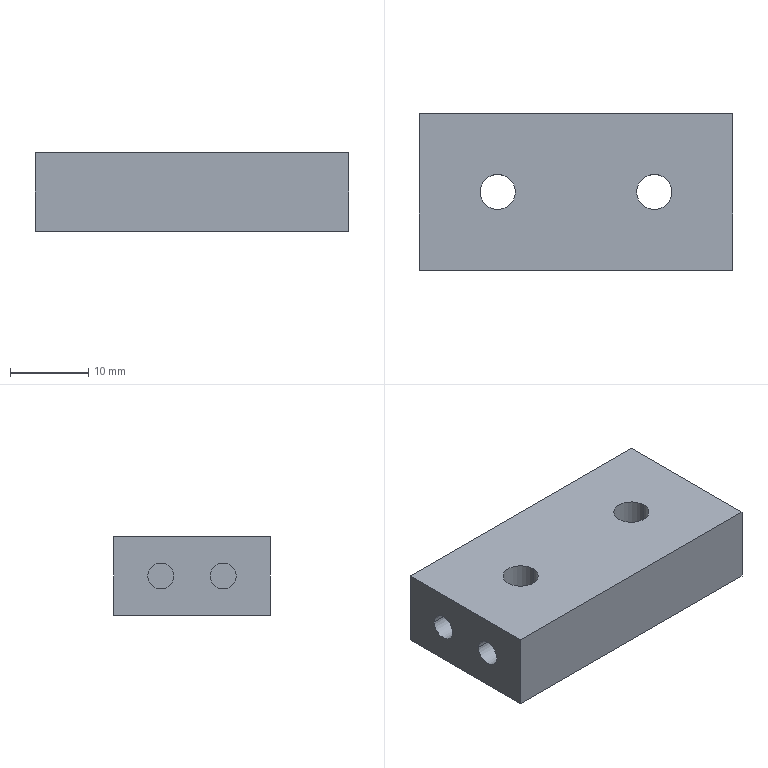Part | SolidWorks | features ICE 2, Extrusion 1 | 1 solid | 22 faces | box 40 x 20 x 10 mm | volume 7288 mm3 | cylinder 12 | plane 10 | commonest cylinder face diameters 3.3 x8 4.5 x4
STEP:
#1=CARTESIAN_POINT('',(9.151,4.195,6.65));
#2=VERTEX_POINT('',#1);
#3=CARTESIAN_POINT('',(9.151,4.195,3.35));
#4=VERTEX_POINT('',#3);
#5=CARTESIAN_POINT('',(9.151,4.195,5.));
#6=DIRECTION('',(1.,0.,0.));
#7=DIRECTION('',(0.,0.,-1.));
#8=AXIS2_PLACEMENT_3D('',#5,#6,#7);
#9=CIRCLE('',#8,1.65);
#10=EDGE_CURVE('',#2,#4,#9,.T.);
#11=ORIENTED_EDGE('',*,*,#10,.F.);
#12=CARTESIAN_POINT('',(20.651,4.195,6.65));
#13=VERTEX_POINT('',#12);
#14=CARTESIAN_POINT('',(9.151,4.195,6.65));
#15=DIRECTION('',(1.,0.,0.));
#16=VECTOR('',#15,1000.);
#17=LINE('',#14,#16);
#18=EDGE_CURVE('',#2,#13,#17,.T.);
#19=ORIENTED_EDGE('',*,*,#18,.T.);
#20=CARTESIAN_POINT('',(20.651,4.195,3.35));
#21=VERTEX_POINT('',#20);
#22=CARTESIAN_POINT('',(20.651,4.195,5.));
#23=DIRECTION('',(1.,0.,0.));
#24=DIRECTION('',(0.,0.,-1.));
#25=AXIS2_PLACEMENT_3D('',#22,#23,#24);
#26=CIRCLE('',#25,1.65);
#27=EDGE_CURVE('',#13,#21,#26,.T.);
#28=ORIENTED_EDGE('',*,*,#27,.T.);
#29=CARTESIAN_POINT('',(9.151,4.195,3.35));
#30=DIRECTION('',(1.,0.,0.));
#31=VECTOR('',#30,1000.);
#32=LINE('',#29,#31);
#33=EDGE_CURVE('',#4,#21,#32,.T.);
#34=ORIENTED_EDGE('',*,*,#33,.F.);
#35=EDGE_LOOP('',(#11,#19,#28,#34));
#36=FACE_OUTER_BOUND('',#35,.T.);
#37=CARTESIAN_POINT('',(9.151,4.195,5.));
#38=DIRECTION('',(1.,0.,0.));
#39=DIRECTION('',(0.,0.,-1.));
#40=AXIS2_PLACEMENT_3D('',#37,#38,#39);
#41=CYLINDRICAL_SURFACE('',#40,1.65);
#42=ADVANCED_FACE('',(#36),#41,.F.);
#43=CARTESIAN_POINT('',(9.151,-3.805,6.65));
#44=VERTEX_POINT('',#43);
#45=CARTESIAN_POINT('',(9.151,-3.805,3.35));
#46=VERTEX_POINT('',#45);
#47=CARTESIAN_POINT('',(9.151,-3.805,5.));
#48=DIRECTION('',(1.,0.,0.));
#49=DIRECTION('',(0.,0.,-1.));
#50=AXIS2_PLACEMENT_3D('',#47,#48,#49);
#51=CIRCLE('',#50,1.65);
#52=EDGE_CURVE('',#44,#46,#51,.T.);
#53=ORIENTED_EDGE('',*,*,#52,.F.);
#54=CARTESIAN_POINT('',(20.651,-3.805,6.65));
#55=VERTEX_POINT('',#54);
#56=CARTESIAN_POINT('',(9.151,-3.805,6.65));
#57=DIRECTION('',(1.,0.,0.));
#58=VECTOR('',#57,1000.);
#59=LINE('',#56,#58);
#60=EDGE_CURVE('',#44,#55,#59,.T.);
#61=ORIENTED_EDGE('',*,*,#60,.T.);
#62=CARTESIAN_POINT('',(20.651,-3.805,3.35));
#63=VERTEX_POINT('',#62);
#64=CARTESIAN_POINT('',(20.651,-3.805,5.));
#65=DIRECTION('',(1.,0.,0.));
#66=DIRECTION('',(0.,0.,-1.));
#67=AXIS2_PLACEMENT_3D('',#64,#65,#66);
#68=CIRCLE('',#67,1.65);
#69=EDGE_CURVE('',#55,#63,#68,.T.);
#70=ORIENTED_EDGE('',*,*,#69,.T.);
#71=CARTESIAN_POINT('',(9.151,-3.805,3.35));
#72=DIRECTION('',(1.,0.,0.));
#73=VECTOR('',#72,1000.);
#74=LINE('',#71,#73);
#75=EDGE_CURVE('',#46,#63,#74,.T.);
#76=ORIENTED_EDGE('',*,*,#75,.F.);
#77=EDGE_LOOP('',(#53,#61,#70,#76));
#78=FACE_OUTER_BOUND('',#77,.T.);
#79=CARTESIAN_POINT('',(9.151,-3.805,5.));
#80=DIRECTION('',(1.,0.,0.));
#81=DIRECTION('',(0.,0.,-1.));
#82=AXIS2_PLACEMENT_3D('',#79,#80,#81);
#83=CYLINDRICAL_SURFACE('',#82,1.65);
#84=ADVANCED_FACE('',(#78),#83,.F.);
#85=CARTESIAN_POINT('',(-7.849,5.845,5.));
#86=VERTEX_POINT('',#85);
#87=CARTESIAN_POINT('',(-7.849,2.545,5.));
#88=VERTEX_POINT('',#87);
#89=CARTESIAN_POINT('',(-7.849,4.195,5.));
#90=DIRECTION('',(-1.,0.,0.));
#91=DIRECTION('',(0.,-1.,0.));
#92=AXIS2_PLACEMENT_3D('',#89,#90,#91);
#93=CIRCLE('',#92,1.65);
#94=EDGE_CURVE('',#86,#88,#93,.T.);
#95=ORIENTED_EDGE('',*,*,#94,.F.);
#96=CARTESIAN_POINT('',(-19.349,5.845,5.));
#97=VERTEX_POINT('',#96);
#98=CARTESIAN_POINT('',(-7.849,5.845,5.));
#99=DIRECTION('',(-1.,0.,0.));
#100=VECTOR('',#99,1000.);
#101=LINE('',#98,#100);
#102=EDGE_CURVE('',#86,#97,#101,.T.);
#103=ORIENTED_EDGE('',*,*,#102,.T.);
#104=CARTESIAN_POINT('',(-19.349,2.545,5.));
#105=VERTEX_POINT('',#104);
#106=CARTESIAN_POINT('',(-19.349,4.195,5.));
#107=DIRECTION('',(-1.,0.,0.));
#108=DIRECTION('',(0.,-1.,0.));
#109=AXIS2_PLACEMENT_3D('',#106,#107,#108);
#110=CIRCLE('',#109,1.65);
#111=EDGE_CURVE('',#97,#105,#110,.T.);
#112=ORIENTED_EDGE('',*,*,#111,.T.);
#113=CARTESIAN_POINT('',(-7.849,2.545,5.));
#114=DIRECTION('',(-1.,0.,0.));
#115=VECTOR('',#114,1000.);
#116=LINE('',#113,#115);
#117=EDGE_CURVE('',#88,#105,#116,.T.);
#118=ORIENTED_EDGE('',*,*,#117,.F.);
#119=EDGE_LOOP('',(#95,#103,#112,#118));
#120=FACE_OUTER_BOUND('',#119,.T.);
#121=CARTESIAN_POINT('',(-7.849,4.195,5.));
#122=DIRECTION('',(-1.,0.,0.));
#123=DIRECTION('',(0.,-1.,0.));
#124=AXIS2_PLACEMENT_3D('',#121,#122,#123);
#125=CYLINDRICAL_SURFACE('',#124,1.65);
#126=ADVANCED_FACE('',(#120),#125,.F.);
#127=CARTESIAN_POINT('',(-7.849,-2.155,5.));
#128=VERTEX_POINT('',#127);
#129=CARTESIAN_POINT('',(-7.849,-5.455,5.));
#130=VERTEX_POINT('',#129);
#131=CARTESIAN_POINT('',(-7.849,-3.805,5.));
#132=DIRECTION('',(-1.,0.,0.));
#133=DIRECTION('',(0.,-1.,0.));
#134=AXIS2_PLACEMENT_3D('',#131,#132,#133);
#135=CIRCLE('',#134,1.65);
#136=EDGE_CURVE('',#128,#130,#135,.T.);
#137=ORIENTED_EDGE('',*,*,#136,.F.);
#138=CARTESIAN_POINT('',(-19.349,-2.155,5.));
#139=VERTEX_POINT('',#138);
#140=CARTESIAN_POINT('',(-7.849,-2.155,5.));
#141=DIRECTION('',(-1.,0.,0.));
#142=VECTOR('',#141,1000.);
#143=LINE('',#140,#142);
#144=EDGE_CURVE('',#128,#139,#143,.T.);
#145=ORIENTED_EDGE('',*,*,#144,.T.);
#146=CARTESIAN_POINT('',(-19.349,-5.455,5.));
#147=VERTEX_POINT('',#146);
#148=CARTESIAN_POINT('',(-19.349,-3.805,5.));
#149=DIRECTION('',(-1.,0.,0.));
#150=DIRECTION('',(0.,-1.,0.));
#151=AXIS2_PLACEMENT_3D('',#148,#149,#150);
#152=CIRCLE('',#151,1.65);
#153=EDGE_CURVE('',#139,#147,#152,.T.);
#154=ORIENTED_EDGE('',*,*,#153,.T.);
#155=CARTESIAN_POINT('',(-7.849,-5.455,5.));
#156=DIRECTION('',(-1.,0.,0.));
#157=VECTOR('',#156,1000.);
#158=LINE('',#155,#157);
#159=EDGE_CURVE('',#130,#147,#158,.T.);
#160=ORIENTED_EDGE('',*,*,#159,.F.);
#161=EDGE_LOOP('',(#137,#145,#154,#160));
#162=FACE_OUTER_BOUND('',#161,.T.);
#163=CARTESIAN_POINT('',(-7.849,-3.805,5.));
#164=DIRECTION('',(-1.,0.,0.));
#165=DIRECTION('',(0.,-1.,0.));
#166=AXIS2_PLACEMENT_3D('',#163,#164,#165);
#167=CYLINDRICAL_SURFACE('',#166,1.65);
#168=ADVANCED_FACE('',(#162),#167,.F.);
#169=CARTESIAN_POINT('',(8.401,0.1954,10.));
#170=VERTEX_POINT('',#169);
#171=CARTESIAN_POINT('',(12.901,0.1954,10.));
#172=VERTEX_POINT('',#171);
#173=CARTESIAN_POINT('',(10.651,0.1954,10.));
#174=DIRECTION('',(0.,0.,1.));
#175=DIRECTION('',(1.,0.,0.));
#176=AXIS2_PLACEMENT_3D('',#173,#174,#175);
#177=CIRCLE('',#176,2.25);
#178=EDGE_CURVE('',#170,#172,#177,.T.);
#179=ORIENTED_EDGE('',*,*,#178,.T.);
#180=CARTESIAN_POINT('',(12.901,0.1954,0.));
#181=VERTEX_POINT('',#180);
#182=CARTESIAN_POINT('',(12.901,0.1954,10.));
#183=DIRECTION('',(0.,0.,-1.));
#184=VECTOR('',#183,1000.);
#185=LINE('',#182,#184);
#186=EDGE_CURVE('',#172,#181,#185,.T.);
#187=ORIENTED_EDGE('',*,*,#186,.T.);
#188=CARTESIAN_POINT('',(8.401,0.1954,0.));
#189=VERTEX_POINT('',#188);
#190=CARTESIAN_POINT('',(10.651,0.1954,0.));
#191=DIRECTION('',(0.,0.,1.));
#192=DIRECTION('',(1.,0.,0.));
#193=AXIS2_PLACEMENT_3D('',#190,#191,#192);
#194=CIRCLE('',#193,2.25);
#195=EDGE_CURVE('',#189,#181,#194,.T.);
#196=ORIENTED_EDGE('',*,*,#195,.F.);
#197=CARTESIAN_POINT('',(8.401,0.1954,10.));
#198=DIRECTION('',(0.,0.,-1.));
#199=VECTOR('',#198,1000.);
#200=LINE('',#197,#199);
#201=EDGE_CURVE('',#170,#189,#200,.T.);
#202=ORIENTED_EDGE('',*,*,#201,.F.);
#203=EDGE_LOOP('',(#179,#187,#196,#202));
#204=FACE_OUTER_BOUND('',#203,.T.);
#205=CARTESIAN_POINT('',(10.651,0.1954,10.));
#206=DIRECTION('',(0.,0.,-1.));
#207=DIRECTION('',(-1.,0.,0.));
#208=AXIS2_PLACEMENT_3D('',#205,#206,#207);
#209=CYLINDRICAL_SURFACE('',#208,2.25);
#210=ADVANCED_FACE('',(#204),#209,.F.);
#211=CARTESIAN_POINT('',(-11.599,0.1954,10.));
#212=VERTEX_POINT('',#211);
#213=CARTESIAN_POINT('',(-7.099,0.1954,10.));
#214=VERTEX_POINT('',#213);
#215=CARTESIAN_POINT('',(-9.349,0.1954,10.));
#216=DIRECTION('',(0.,0.,1.));
#217=DIRECTION('',(1.,0.,0.));
#218=AXIS2_PLACEMENT_3D('',#215,#216,#217);
#219=CIRCLE('',#218,2.25);
#220=EDGE_CURVE('',#212,#214,#219,.T.);
#221=ORIENTED_EDGE('',*,*,#220,.T.);
#222=CARTESIAN_POINT('',(-7.099,0.1954,0.));
#223=VERTEX_POINT('',#222);
#224=CARTESIAN_POINT('',(-7.099,0.1954,10.));
#225=DIRECTION('',(0.,0.,-1.));
#226=VECTOR('',#225,1000.);
#227=LINE('',#224,#226);
#228=EDGE_CURVE('',#214,#223,#227,.T.);
#229=ORIENTED_EDGE('',*,*,#228,.T.);
#230=CARTESIAN_POINT('',(-11.599,0.1954,0.));
#231=VERTEX_POINT('',#230);
#232=CARTESIAN_POINT('',(-9.349,0.1954,0.));
#233=DIRECTION('',(0.,0.,1.));
#234=DIRECTION('',(1.,0.,0.));
#235=AXIS2_PLACEMENT_3D('',#232,#233,#234);
#236=CIRCLE('',#235,2.25);
#237=EDGE_CURVE('',#231,#223,#236,.T.);
#238=ORIENTED_EDGE('',*,*,#237,.F.);
#239=CARTESIAN_POINT('',(-11.599,0.1954,10.));
#240=DIRECTION('',(0.,0.,-1.));
#241=VECTOR('',#240,1000.);
#242=LINE('',#239,#241);
#243=EDGE_CURVE('',#212,#231,#242,.T.);
#244=ORIENTED_EDGE('',*,*,#243,.F.);
#245=EDGE_LOOP('',(#221,#229,#238,#244));
#246=FACE_OUTER_BOUND('',#245,.T.);
#247=CARTESIAN_POINT('',(-9.349,0.1954,10.));
#248=DIRECTION('',(0.,0.,-1.));
#249=DIRECTION('',(-1.,0.,0.));
#250=AXIS2_PLACEMENT_3D('',#247,#248,#249);
#251=CYLINDRICAL_SURFACE('',#250,2.25);
#252=ADVANCED_FACE('',(#246),#251,.F.);
#253=ORIENTED_EDGE('',*,*,#220,.F.);
#254=CARTESIAN_POINT('',(-9.349,0.1954,10.));
#255=DIRECTION('',(0.,0.,1.));
#256=DIRECTION('',(1.,0.,0.));
#257=AXIS2_PLACEMENT_3D('',#254,#255,#256);
#258=CIRCLE('',#257,2.25);
#259=EDGE_CURVE('',#214,#212,#258,.T.);
#260=ORIENTED_EDGE('',*,*,#259,.F.);
#261=EDGE_LOOP('',(#253,#260));
#262=FACE_BOUND('',#261,.T.);
#263=CARTESIAN_POINT('',(-19.349,10.195,10.));
#264=VERTEX_POINT('',#263);
#265=CARTESIAN_POINT('',(-19.349,-9.805,10.));
#266=VERTEX_POINT('',#265);
#267=CARTESIAN_POINT('',(-19.349,10.195,10.));
#268=DIRECTION('',(0.,-1.,0.));
#269=VECTOR('',#268,1000.);
#270=LINE('',#267,#269);
#271=EDGE_CURVE('',#264,#266,#270,.T.);
#272=ORIENTED_EDGE('',*,*,#271,.T.);
#273=CARTESIAN_POINT('',(20.651,-9.805,10.));
#274=VERTEX_POINT('',#273);
#275=CARTESIAN_POINT('',(-19.349,-9.805,10.));
#276=DIRECTION('',(1.,0.,0.));
#277=VECTOR('',#276,1000.);
#278=LINE('',#275,#277);
#279=EDGE_CURVE('',#266,#274,#278,.T.);
#280=ORIENTED_EDGE('',*,*,#279,.T.);
#281=CARTESIAN_POINT('',(20.651,10.195,10.));
#282=VERTEX_POINT('',#281);
#283=CARTESIAN_POINT('',(20.651,10.195,10.));
#284=DIRECTION('',(0.,1.,0.));
#285=VECTOR('',#284,1000.);
#286=LINE('',#283,#285);
#287=EDGE_CURVE('',#274,#282,#286,.T.);
#288=ORIENTED_EDGE('',*,*,#287,.T.);
#289=CARTESIAN_POINT('',(-19.349,10.195,10.));
#290=DIRECTION('',(-1.,0.,0.));
#291=VECTOR('',#290,1000.);
#292=LINE('',#289,#291);
#293=EDGE_CURVE('',#282,#264,#292,.T.);
#294=ORIENTED_EDGE('',*,*,#293,.T.);
#295=EDGE_LOOP('',(#272,#280,#288,#294));
#296=FACE_OUTER_BOUND('',#295,.T.);
#297=ORIENTED_EDGE('',*,*,#178,.F.);
#298=CARTESIAN_POINT('',(10.651,0.1954,10.));
#299=DIRECTION('',(0.,0.,1.));
#300=DIRECTION('',(1.,0.,0.));
#301=AXIS2_PLACEMENT_3D('',#298,#299,#300);
#302=CIRCLE('',#301,2.25);
#303=EDGE_CURVE('',#172,#170,#302,.T.);
#304=ORIENTED_EDGE('',*,*,#303,.F.);
#305=EDGE_LOOP('',(#297,#304));
#306=FACE_BOUND('',#305,.T.);
#307=CARTESIAN_POINT('',(0.,0.,10.));
#308=DIRECTION('',(0.,0.,1.));
#309=DIRECTION('',(1.,0.,0.));
#310=AXIS2_PLACEMENT_3D('',#307,#308,#309);
#311=PLANE('',#310);
#312=ADVANCED_FACE('',(#262,#296,#306),#311,.T.);
#313=CARTESIAN_POINT('',(-19.349,10.195,0.));
#314=VERTEX_POINT('',#313);
#315=CARTESIAN_POINT('',(-19.349,-9.805,0.));
#316=VERTEX_POINT('',#315);
#317=CARTESIAN_POINT('',(-19.349,10.195,0.));
#318=DIRECTION('',(0.,-1.,0.));
#319=VECTOR('',#318,1000.);
#320=LINE('',#317,#319);
#321=EDGE_CURVE('',#314,#316,#320,.T.);
#322=ORIENTED_EDGE('',*,*,#321,.F.);
#323=CARTESIAN_POINT('',(20.651,10.195,0.));
#324=VERTEX_POINT('',#323);
#325=CARTESIAN_POINT('',(-19.349,10.195,0.));
#326=DIRECTION('',(-1.,0.,0.));
#327=VECTOR('',#326,1000.);
#328=LINE('',#325,#327);
#329=EDGE_CURVE('',#324,#314,#328,.T.);
#330=ORIENTED_EDGE('',*,*,#329,.F.);
#331=CARTESIAN_POINT('',(20.651,-9.805,0.));
#332=VERTEX_POINT('',#331);
#333=CARTESIAN_POINT('',(20.651,10.195,0.));
#334=DIRECTION('',(0.,1.,0.));
#335=VECTOR('',#334,1000.);
#336=LINE('',#333,#335);
#337=EDGE_CURVE('',#332,#324,#336,.T.);
#338=ORIENTED_EDGE('',*,*,#337,.F.);
#339=CARTESIAN_POINT('',(-19.349,-9.805,0.));
#340=DIRECTION('',(1.,0.,0.));
#341=VECTOR('',#340,1000.);
#342=LINE('',#339,#341);
#343=EDGE_CURVE('',#316,#332,#342,.T.);
#344=ORIENTED_EDGE('',*,*,#343,.F.);
#345=EDGE_LOOP('',(#322,#330,#338,#344));
#346=FACE_OUTER_BOUND('',#345,.T.);
#347=ORIENTED_EDGE('',*,*,#237,.T.);
#348=CARTESIAN_POINT('',(-9.349,0.1954,0.));
#349=DIRECTION('',(0.,0.,1.));
#350=DIRECTION('',(1.,0.,0.));
#351=AXIS2_PLACEMENT_3D('',#348,#349,#350);
#352=CIRCLE('',#351,2.25);
#353=EDGE_CURVE('',#223,#231,#352,.T.);
#354=ORIENTED_EDGE('',*,*,#353,.T.);
#355=EDGE_LOOP('',(#347,#354));
#356=FACE_BOUND('',#355,.T.);
#357=ORIENTED_EDGE('',*,*,#195,.T.);
#358=CARTESIAN_POINT('',(10.651,0.1954,0.));
#359=DIRECTION('',(0.,0.,1.));
#360=DIRECTION('',(1.,0.,0.));
#361=AXIS2_PLACEMENT_3D('',#358,#359,#360);
#362=CIRCLE('',#361,2.25);
#363=EDGE_CURVE('',#181,#189,#362,.T.);
#364=ORIENTED_EDGE('',*,*,#363,.T.);
#365=EDGE_LOOP('',(#357,#364));
#366=FACE_BOUND('',#365,.T.);
#367=CARTESIAN_POINT('',(0.,0.,0.));
#368=DIRECTION('',(0.,0.,1.));
#369=DIRECTION('',(1.,0.,0.));
#370=AXIS2_PLACEMENT_3D('',#367,#368,#369);
#371=PLANE('',#370);
#372=ADVANCED_FACE('',(#346,#356,#366),#371,.F.);
#373=CARTESIAN_POINT('',(-19.349,4.195,5.));
#374=DIRECTION('',(-1.,0.,0.));
#375=DIRECTION('',(0.,-1.,0.));
#376=AXIS2_PLACEMENT_3D('',#373,#374,#375);
#377=CIRCLE('',#376,1.65);
#378=EDGE_CURVE('',#105,#97,#377,.T.);
#379=ORIENTED_EDGE('',*,*,#378,.F.);
#380=ORIENTED_EDGE('',*,*,#111,.F.);
#381=EDGE_LOOP('',(#379,#380));
#382=FACE_BOUND('',#381,.T.);
#383=CARTESIAN_POINT('',(-19.349,-3.805,5.));
#384=DIRECTION('',(-1.,0.,0.));
#385=DIRECTION('',(0.,-1.,0.));
#386=AXIS2_PLACEMENT_3D('',#383,#384,#385);
#387=CIRCLE('',#386,1.65);
#388=EDGE_CURVE('',#147,#139,#387,.T.);
#389=ORIENTED_EDGE('',*,*,#388,.F.);
#390=ORIENTED_EDGE('',*,*,#153,.F.);
#391=EDGE_LOOP('',(#389,#390));
#392=FACE_BOUND('',#391,.T.);
#393=ORIENTED_EDGE('',*,*,#321,.T.);
#394=CARTESIAN_POINT('',(-19.349,-9.805,10.));
#395=DIRECTION('',(0.,0.,-1.));
#396=VECTOR('',#395,1000.);
#397=LINE('',#394,#396);
#398=EDGE_CURVE('',#266,#316,#397,.T.);
#399=ORIENTED_EDGE('',*,*,#398,.F.);
#400=ORIENTED_EDGE('',*,*,#271,.F.);
#401=CARTESIAN_POINT('',(-19.349,10.195,10.));
#402=DIRECTION('',(0.,0.,-1.));
#403=VECTOR('',#402,1000.);
#404=LINE('',#401,#403);
#405=EDGE_CURVE('',#264,#314,#404,.T.);
#406=ORIENTED_EDGE('',*,*,#405,.T.);
#407=EDGE_LOOP('',(#393,#399,#400,#406));
#408=FACE_OUTER_BOUND('',#407,.T.);
#409=CARTESIAN_POINT('',(-19.349,10.195,10.));
#410=DIRECTION('',(1.,0.,0.));
#411=DIRECTION('',(0.,1.,0.));
#412=AXIS2_PLACEMENT_3D('',#409,#410,#411);
#413=PLANE('',#412);
#414=ADVANCED_FACE('',(#382,#392,#408),#413,.F.);
#415=ORIENTED_EDGE('',*,*,#343,.T.);
#416=CARTESIAN_POINT('',(20.651,-9.805,10.));
#417=DIRECTION('',(0.,0.,-1.));
#418=VECTOR('',#417,1000.);
#419=LINE('',#416,#418);
#420=EDGE_CURVE('',#274,#332,#419,.T.);
#421=ORIENTED_EDGE('',*,*,#420,.F.);
#422=ORIENTED_EDGE('',*,*,#279,.F.);
#423=ORIENTED_EDGE('',*,*,#398,.T.);
#424=EDGE_LOOP('',(#415,#421,#422,#423));
#425=FACE_OUTER_BOUND('',#424,.T.);
#426=CARTESIAN_POINT('',(-19.349,-9.805,10.));
#427=DIRECTION('',(0.,1.,0.));
#428=DIRECTION('',(0.,0.,1.));
#429=AXIS2_PLACEMENT_3D('',#426,#427,#428);
#430=PLANE('',#429);
#431=ADVANCED_FACE('',(#425),#430,.F.);
#432=CARTESIAN_POINT('',(20.651,4.195,5.));
#433=DIRECTION('',(1.,0.,0.));
#434=DIRECTION('',(0.,0.,-1.));
#435=AXIS2_PLACEMENT_3D('',#432,#433,#434);
#436=CIRCLE('',#435,1.65);
#437=EDGE_CURVE('',#21,#13,#436,.T.);
#438=ORIENTED_EDGE('',*,*,#437,.F.);
#439=ORIENTED_EDGE('',*,*,#27,.F.);
#440=EDGE_LOOP('',(#438,#439));
#441=FACE_BOUND('',#440,.T.);
#442=CARTESIAN_POINT('',(20.651,-3.805,5.));
#443=DIRECTION('',(1.,0.,0.));
#444=DIRECTION('',(0.,0.,-1.));
#445=AXIS2_PLACEMENT_3D('',#442,#443,#444);
#446=CIRCLE('',#445,1.65);
#447=EDGE_CURVE('',#63,#55,#446,.T.);
#448=ORIENTED_EDGE('',*,*,#447,.F.);
#449=ORIENTED_EDGE('',*,*,#69,.F.);
#450=EDGE_LOOP('',(#448,#449));
#451=FACE_BOUND('',#450,.T.);
#452=ORIENTED_EDGE('',*,*,#337,.T.);
#453=CARTESIAN_POINT('',(20.651,10.195,10.));
#454=DIRECTION('',(0.,0.,-1.));
#455=VECTOR('',#454,1000.);
#456=LINE('',#453,#455);
#457=EDGE_CURVE('',#282,#324,#456,.T.);
#458=ORIENTED_EDGE('',*,*,#457,.F.);
#459=ORIENTED_EDGE('',*,*,#287,.F.);
#460=ORIENTED_EDGE('',*,*,#420,.T.);
#461=EDGE_LOOP('',(#452,#458,#459,#460));
#462=FACE_OUTER_BOUND('',#461,.T.);
#463=CARTESIAN_POINT('',(20.651,10.195,10.));
#464=DIRECTION('',(-1.,0.,0.));
#465=DIRECTION('',(0.,0.,1.));
#466=AXIS2_PLACEMENT_3D('',#463,#464,#465);
#467=PLANE('',#466);
#468=ADVANCED_FACE('',(#441,#451,#462),#467,.F.);
#469=ORIENTED_EDGE('',*,*,#329,.T.);
#470=ORIENTED_EDGE('',*,*,#405,.F.);
#471=ORIENTED_EDGE('',*,*,#293,.F.);
#472=ORIENTED_EDGE('',*,*,#457,.T.);
#473=EDGE_LOOP('',(#469,#470,#471,#472));
#474=FACE_OUTER_BOUND('',#473,.T.);
#475=CARTESIAN_POINT('',(-19.349,10.195,10.));
#476=DIRECTION('',(0.,-1.,0.));
#477=DIRECTION('',(0.,0.,-1.));
#478=AXIS2_PLACEMENT_3D('',#475,#476,#477);
#479=PLANE('',#478);
#480=ADVANCED_FACE('',(#474),#479,.F.);
#481=ORIENTED_EDGE('',*,*,#228,.F.);
#482=ORIENTED_EDGE('',*,*,#259,.T.);
#483=ORIENTED_EDGE('',*,*,#243,.T.);
#484=ORIENTED_EDGE('',*,*,#353,.F.);
#485=EDGE_LOOP('',(#481,#482,#483,#484));
#486=FACE_OUTER_BOUND('',#485,.T.);
#487=CARTESIAN_POINT('',(-9.349,0.1954,10.));
#488=DIRECTION('',(0.,0.,-1.));
#489=DIRECTION('',(-1.,0.,0.));
#490=AXIS2_PLACEMENT_3D('',#487,#488,#489);
#491=CYLINDRICAL_SURFACE('',#490,2.25);
#492=ADVANCED_FACE('',(#486),#491,.F.);
#493=ORIENTED_EDGE('',*,*,#186,.F.);
#494=ORIENTED_EDGE('',*,*,#303,.T.);
#495=ORIENTED_EDGE('',*,*,#201,.T.);
#496=ORIENTED_EDGE('',*,*,#363,.F.);
#497=EDGE_LOOP('',(#493,#494,#495,#496));
#498=FACE_OUTER_BOUND('',#497,.T.);
#499=CARTESIAN_POINT('',(10.651,0.1954,10.));
#500=DIRECTION('',(0.,0.,-1.));
#501=DIRECTION('',(-1.,0.,0.));
#502=AXIS2_PLACEMENT_3D('',#499,#500,#501);
#503=CYLINDRICAL_SURFACE('',#502,2.25);
#504=ADVANCED_FACE('',(#498),#503,.F.);
#505=ORIENTED_EDGE('',*,*,#144,.F.);
#506=CARTESIAN_POINT('',(-7.849,-3.805,5.));
#507=DIRECTION('',(-1.,0.,0.));
#508=DIRECTION('',(0.,-1.,0.));
#509=AXIS2_PLACEMENT_3D('',#506,#507,#508);
#510=CIRCLE('',#509,1.65);
#511=EDGE_CURVE('',#130,#128,#510,.T.);
#512=ORIENTED_EDGE('',*,*,#511,.F.);
#513=ORIENTED_EDGE('',*,*,#159,.T.);
#514=ORIENTED_EDGE('',*,*,#388,.T.);
#515=EDGE_LOOP('',(#505,#512,#513,#514));
#516=FACE_OUTER_BOUND('',#515,.T.);
#517=CARTESIAN_POINT('',(-7.849,-3.805,5.));
#518=DIRECTION('',(-1.,0.,0.));
#519=DIRECTION('',(0.,-1.,0.));
#520=AXIS2_PLACEMENT_3D('',#517,#518,#519);
#521=CYLINDRICAL_SURFACE('',#520,1.65);
#522=ADVANCED_FACE('',(#516),#521,.F.);
#523=ORIENTED_EDGE('',*,*,#511,.T.);
#524=ORIENTED_EDGE('',*,*,#136,.T.);
#525=EDGE_LOOP('',(#523,#524));
#526=FACE_OUTER_BOUND('',#525,.T.);
#527=CARTESIAN_POINT('',(-7.849,-3.805,5.));
#528=DIRECTION('',(-1.,0.,0.));
#529=DIRECTION('',(0.,-1.,0.));
#530=AXIS2_PLACEMENT_3D('',#527,#528,#529);
#531=PLANE('',#530);
#532=ADVANCED_FACE('',(#526),#531,.T.);
#533=ORIENTED_EDGE('',*,*,#102,.F.);
#534=CARTESIAN_POINT('',(-7.849,4.195,5.));
#535=DIRECTION('',(-1.,0.,0.));
#536=DIRECTION('',(0.,-1.,0.));
#537=AXIS2_PLACEMENT_3D('',#534,#535,#536);
#538=CIRCLE('',#537,1.65);
#539=EDGE_CURVE('',#88,#86,#538,.T.);
#540=ORIENTED_EDGE('',*,*,#539,.F.);
#541=ORIENTED_EDGE('',*,*,#117,.T.);
#542=ORIENTED_EDGE('',*,*,#378,.T.);
#543=EDGE_LOOP('',(#533,#540,#541,#542));
#544=FACE_OUTER_BOUND('',#543,.T.);
#545=CARTESIAN_POINT('',(-7.849,4.195,5.));
#546=DIRECTION('',(-1.,0.,0.));
#547=DIRECTION('',(0.,-1.,0.));
#548=AXIS2_PLACEMENT_3D('',#545,#546,#547);
#549=CYLINDRICAL_SURFACE('',#548,1.65);
#550=ADVANCED_FACE('',(#544),#549,.F.);
#551=ORIENTED_EDGE('',*,*,#539,.T.);
#552=ORIENTED_EDGE('',*,*,#94,.T.);
#553=EDGE_LOOP('',(#551,#552));
#554=FACE_OUTER_BOUND('',#553,.T.);
#555=CARTESIAN_POINT('',(-7.849,4.195,5.));
#556=DIRECTION('',(-1.,0.,0.));
#557=DIRECTION('',(0.,-1.,0.));
#558=AXIS2_PLACEMENT_3D('',#555,#556,#557);
#559=PLANE('',#558);
#560=ADVANCED_FACE('',(#554),#559,.T.);
#561=ORIENTED_EDGE('',*,*,#60,.F.);
#562=CARTESIAN_POINT('',(9.151,-3.805,5.));
#563=DIRECTION('',(1.,0.,0.));
#564=DIRECTION('',(0.,0.,-1.));
#565=AXIS2_PLACEMENT_3D('',#562,#563,#564);
#566=CIRCLE('',#565,1.65);
#567=EDGE_CURVE('',#46,#44,#566,.T.);
#568=ORIENTED_EDGE('',*,*,#567,.F.);
#569=ORIENTED_EDGE('',*,*,#75,.T.);
#570=ORIENTED_EDGE('',*,*,#447,.T.);
#571=EDGE_LOOP('',(#561,#568,#569,#570));
#572=FACE_OUTER_BOUND('',#571,.T.);
#573=CARTESIAN_POINT('',(9.151,-3.805,5.));
#574=DIRECTION('',(1.,0.,0.));
#575=DIRECTION('',(0.,0.,-1.));
#576=AXIS2_PLACEMENT_3D('',#573,#574,#575);
#577=CYLINDRICAL_SURFACE('',#576,1.65);
#578=ADVANCED_FACE('',(#572),#577,.F.);
#579=ORIENTED_EDGE('',*,*,#567,.T.);
#580=ORIENTED_EDGE('',*,*,#52,.T.);
#581=EDGE_LOOP('',(#579,#580));
#582=FACE_OUTER_BOUND('',#581,.T.);
#583=CARTESIAN_POINT('',(9.151,-3.805,5.));
#584=DIRECTION('',(1.,0.,0.));
#585=DIRECTION('',(0.,0.,-1.));
#586=AXIS2_PLACEMENT_3D('',#583,#584,#585);
#587=PLANE('',#586);
#588=ADVANCED_FACE('',(#582),#587,.T.);
#589=ORIENTED_EDGE('',*,*,#18,.F.);
#590=CARTESIAN_POINT('',(9.151,4.195,5.));
#591=DIRECTION('',(1.,0.,0.));
#592=DIRECTION('',(0.,0.,-1.));
#593=AXIS2_PLACEMENT_3D('',#590,#591,#592);
#594=CIRCLE('',#593,1.65);
#595=EDGE_CURVE('',#4,#2,#594,.T.);
#596=ORIENTED_EDGE('',*,*,#595,.F.);
#597=ORIENTED_EDGE('',*,*,#33,.T.);
#598=ORIENTED_EDGE('',*,*,#437,.T.);
#599=EDGE_LOOP('',(#589,#596,#597,#598));
#600=FACE_OUTER_BOUND('',#599,.T.);
#601=CARTESIAN_POINT('',(9.151,4.195,5.));
#602=DIRECTION('',(1.,0.,0.));
#603=DIRECTION('',(0.,0.,-1.));
#604=AXIS2_PLACEMENT_3D('',#601,#602,#603);
#605=CYLINDRICAL_SURFACE('',#604,1.65);
#606=ADVANCED_FACE('',(#600),#605,.F.);
#607=ORIENTED_EDGE('',*,*,#595,.T.);
#608=ORIENTED_EDGE('',*,*,#10,.T.);
#609=EDGE_LOOP('',(#607,#608));
#610=FACE_OUTER_BOUND('',#609,.T.);
#611=CARTESIAN_POINT('',(9.151,4.195,5.));
#612=DIRECTION('',(1.,0.,0.));
#613=DIRECTION('',(0.,0.,-1.));
#614=AXIS2_PLACEMENT_3D('',#611,#612,#613);
#615=PLANE('',#614);
#616=ADVANCED_FACE('',(#610),#615,.T.);
#617=CLOSED_SHELL('',(#42,#84,#126,#168,#210,#252,#312,#372,#414,#431,#468,#480,#492,#504,#522,#532,#550,#560,#578,#588,#606,#616));
#618=MANIFOLD_SOLID_BREP('',#617);
#619=CARTESIAN_POINT('',(0.,0.,0.));
#620=DIRECTION('',(0.,0.,1.));
#621=DIRECTION('',(1.,0.,0.));
#622=AXIS2_PLACEMENT_3D('',#619,#620,#621);
#623=(LENGTH_UNIT()NAMED_UNIT(*)SI_UNIT(.MILLI.,.METRE.));
#624=UNCERTAINTY_MEASURE_WITH_UNIT(LENGTH_MEASURE(0.00001),#623,'','');
#625=(NAMED_UNIT(*)PLANE_ANGLE_UNIT()SI_UNIT($,.RADIAN.));
#626=(NAMED_UNIT(*)SI_UNIT($,.STERADIAN.)SOLID_ANGLE_UNIT());
#627=(GEOMETRIC_REPRESENTATION_CONTEXT(3)GLOBAL_UNCERTAINTY_ASSIGNED_CONTEXT((#624))GLOBAL_UNIT_ASSIGNED_CONTEXT((#623,#625,#626))REPRESENTATION_CONTEXT('',''));
#628=ADVANCED_BREP_SHAPE_REPRESENTATION('',(#618,#622),#627);